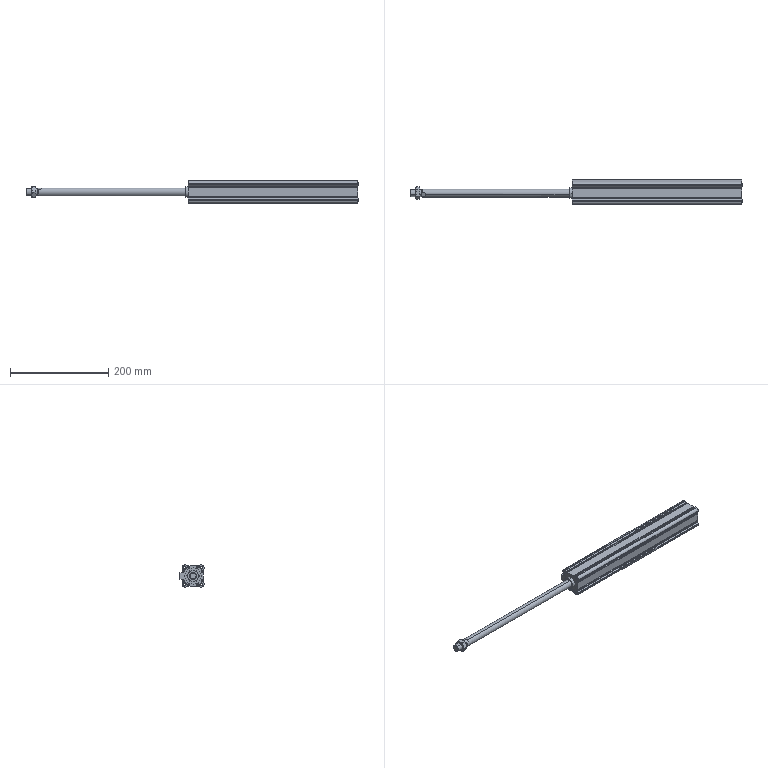Part | SolidWorks | 5 solids | 252 faces | box 676 x 49.5 x 45 mm | volume 398264 mm3 | plane 118 | cylinder 94 | cone 40 | commonest cylinder face diameters 4.26 x18 4.917 x16 0.6 x8 6 x8 4 x6 2 x4